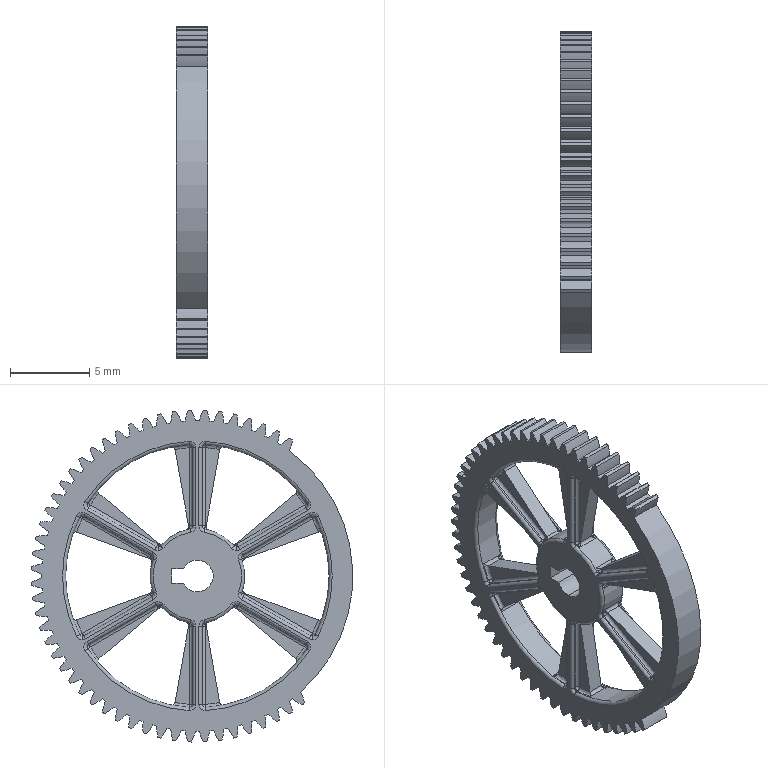Part | SolidWorks | features ICE 4, CirPattern 2, Fillet 2, BaseBody 1, MirrorPattern 1 | 1 solid | 608 faces | box 2 x 20.317 x 20.986 mm | volume 331.893 mm3 | cylinder 351 | torus 132 | plane 65 | sphere 60 | commonest cylinder face diameters 0.4 x138 8.16 x99 19.648 x50 21 x49 6 x6 16.648 x6